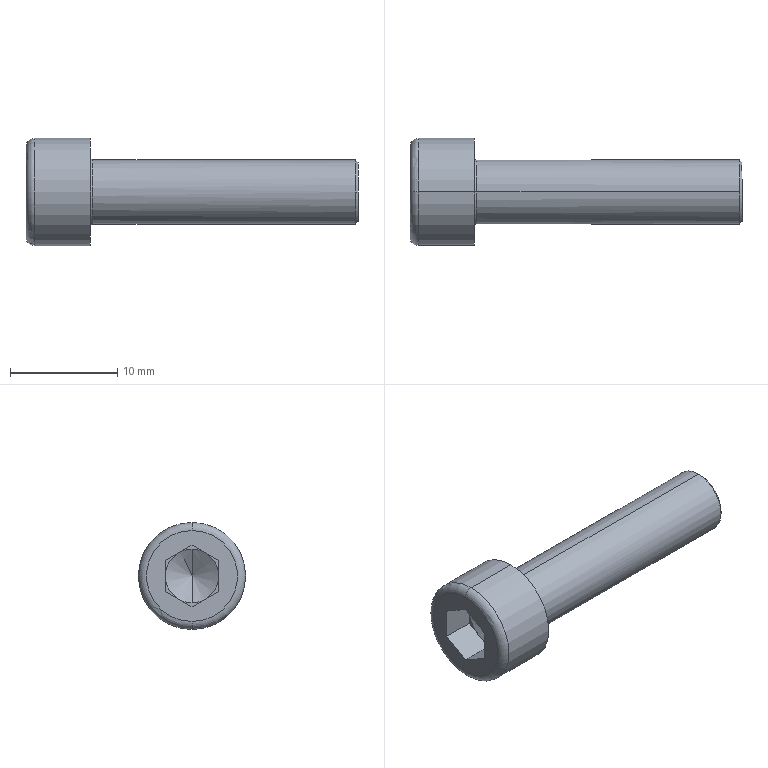Part | SolidWorks | features BaseBody 1 | 1 solid | 27 faces | box 31 x 10 x 10 mm | volume 1100 mm3 | plane 15 | cylinder 4 | cone 4 | torus 4 | commonest cylinder face diameters 6 x2 10 x2
STEP:
#1=CARTESIAN_POINT('',(30.75,3.,0.));
#2=VERTEX_POINT('',#1);
#3=CARTESIAN_POINT('',(30.75,0.,-3.));
#4=VERTEX_POINT('',#3);
#5=CARTESIAN_POINT('',(30.75,0.,0.));
#6=DIRECTION('',(-1.,0.,0.));
#7=DIRECTION('',(0.,0.,1.));
#8=AXIS2_PLACEMENT_3D('',#5,#6,#7);
#9=CIRCLE('',#8,3.);
#10=EDGE_CURVE('',#2,#4,#9,.T.);
#11=ORIENTED_EDGE('',*,*,#10,.T.);
#12=CARTESIAN_POINT('',(6.25,0.,-3.));
#13=VERTEX_POINT('',#12);
#14=CARTESIAN_POINT('',(31.,0.,-3.));
#15=DIRECTION('',(-1.,0.,0.));
#16=VECTOR('',#15,1000.);
#17=LINE('',#14,#16);
#18=EDGE_CURVE('',#4,#13,#17,.T.);
#19=ORIENTED_EDGE('',*,*,#18,.T.);
#20=CARTESIAN_POINT('',(6.25,0.,3.));
#21=VERTEX_POINT('',#20);
#22=CARTESIAN_POINT('',(6.25,0.,0.));
#23=DIRECTION('',(1.,0.,0.));
#24=DIRECTION('',(0.,0.,1.));
#25=AXIS2_PLACEMENT_3D('',#22,#23,#24);
#26=CIRCLE('',#25,3.);
#27=EDGE_CURVE('',#13,#21,#26,.T.);
#28=ORIENTED_EDGE('',*,*,#27,.T.);
#29=CARTESIAN_POINT('',(30.75,0.,3.));
#30=VERTEX_POINT('',#29);
#31=CARTESIAN_POINT('',(31.,0.,3.));
#32=DIRECTION('',(-1.,0.,0.));
#33=VECTOR('',#32,1000.);
#34=LINE('',#31,#33);
#35=EDGE_CURVE('',#30,#21,#34,.T.);
#36=ORIENTED_EDGE('',*,*,#35,.F.);
#37=CARTESIAN_POINT('',(30.75,0.,0.));
#38=DIRECTION('',(-1.,0.,0.));
#39=DIRECTION('',(0.,0.,1.));
#40=AXIS2_PLACEMENT_3D('',#37,#38,#39);
#41=CIRCLE('',#40,3.);
#42=EDGE_CURVE('',#30,#2,#41,.T.);
#43=ORIENTED_EDGE('',*,*,#42,.T.);
#44=EDGE_LOOP('',(#11,#19,#28,#36,#43));
#45=FACE_OUTER_BOUND('',#44,.T.);
#46=CARTESIAN_POINT('',(31.,0.,0.));
#47=DIRECTION('',(-1.,0.,0.));
#48=DIRECTION('',(0.,0.,1.));
#49=AXIS2_PLACEMENT_3D('',#46,#47,#48);
#50=CYLINDRICAL_SURFACE('',#49,3.);
#51=ADVANCED_FACE('',(#45),#50,.T.);
#52=CARTESIAN_POINT('',(31.,-2.75,0.));
#53=VERTEX_POINT('',#52);
#54=CARTESIAN_POINT('',(31.,2.75,0.));
#55=VERTEX_POINT('',#54);
#56=CARTESIAN_POINT('',(31.,0.,0.));
#57=DIRECTION('',(-1.,0.,0.));
#58=DIRECTION('',(0.,-1.,0.));
#59=AXIS2_PLACEMENT_3D('',#56,#57,#58);
#60=CIRCLE('',#59,2.75);
#61=EDGE_CURVE('',#53,#55,#60,.T.);
#62=ORIENTED_EDGE('',*,*,#61,.T.);
#63=CARTESIAN_POINT('',(30.75,3.,0.));
#64=DIRECTION('',(-0.7071,0.7071,0.));
#65=VECTOR('',#64,1000.);
#66=LINE('',#63,#65);
#67=EDGE_CURVE('',#55,#2,#66,.T.);
#68=ORIENTED_EDGE('',*,*,#67,.T.);
#69=ORIENTED_EDGE('',*,*,#42,.F.);
#70=CARTESIAN_POINT('',(30.75,-3.,0.));
#71=VERTEX_POINT('',#70);
#72=CARTESIAN_POINT('',(30.75,0.,0.));
#73=DIRECTION('',(-1.,0.,0.));
#74=DIRECTION('',(0.,0.,1.));
#75=AXIS2_PLACEMENT_3D('',#72,#73,#74);
#76=CIRCLE('',#75,3.);
#77=EDGE_CURVE('',#71,#30,#76,.T.);
#78=ORIENTED_EDGE('',*,*,#77,.F.);
#79=CARTESIAN_POINT('',(30.75,-3.,0.));
#80=DIRECTION('',(-0.7071,-0.7071,0.));
#81=VECTOR('',#80,1000.);
#82=LINE('',#79,#81);
#83=EDGE_CURVE('',#53,#71,#82,.T.);
#84=ORIENTED_EDGE('',*,*,#83,.F.);
#85=EDGE_LOOP('',(#62,#68,#69,#78,#84));
#86=FACE_OUTER_BOUND('',#85,.T.);
#87=CARTESIAN_POINT('',(30.75,0.,0.));
#88=DIRECTION('',(-1.,0.,0.));
#89=DIRECTION('',(0.,-1.,0.));
#90=AXIS2_PLACEMENT_3D('',#87,#88,#89);
#91=CONICAL_SURFACE('',#90,3.,0.7854);
#92=ADVANCED_FACE('',(#86),#91,.T.);
#93=CARTESIAN_POINT('',(6.25,0.,0.));
#94=DIRECTION('',(1.,0.,0.));
#95=DIRECTION('',(0.,0.,1.));
#96=AXIS2_PLACEMENT_3D('',#93,#94,#95);
#97=CIRCLE('',#96,3.);
#98=EDGE_CURVE('',#21,#13,#97,.T.);
#99=ORIENTED_EDGE('',*,*,#98,.F.);
#100=CARTESIAN_POINT('',(6.,0.,3.25));
#101=VERTEX_POINT('',#100);
#102=CARTESIAN_POINT('',(6.25,0.,3.25));
#103=DIRECTION('',(0.,1.,0.));
#104=DIRECTION('',(0.,0.,1.));
#105=AXIS2_PLACEMENT_3D('',#102,#103,#104);
#106=CIRCLE('',#105,0.25);
#107=EDGE_CURVE('',#21,#101,#106,.T.);
#108=ORIENTED_EDGE('',*,*,#107,.T.);
#109=CARTESIAN_POINT('',(6.,0.,-3.25));
#110=VERTEX_POINT('',#109);
#111=CARTESIAN_POINT('',(6.,0.,0.));
#112=DIRECTION('',(-1.,0.,0.));
#113=DIRECTION('',(0.,0.,-1.));
#114=AXIS2_PLACEMENT_3D('',#111,#112,#113);
#115=CIRCLE('',#114,3.25);
#116=EDGE_CURVE('',#110,#101,#115,.T.);
#117=ORIENTED_EDGE('',*,*,#116,.F.);
#118=CARTESIAN_POINT('',(6.25,0.,-3.25));
#119=DIRECTION('',(0.,-1.,0.));
#120=DIRECTION('',(0.,0.,-1.));
#121=AXIS2_PLACEMENT_3D('',#118,#119,#120);
#122=CIRCLE('',#121,0.25);
#123=EDGE_CURVE('',#13,#110,#122,.T.);
#124=ORIENTED_EDGE('',*,*,#123,.F.);
#125=EDGE_LOOP('',(#99,#108,#117,#124));
#126=FACE_OUTER_BOUND('',#125,.T.);
#127=CARTESIAN_POINT('',(6.25,0.,0.));
#128=DIRECTION('',(1.,0.,0.));
#129=DIRECTION('',(0.,0.,-1.));
#130=AXIS2_PLACEMENT_3D('',#127,#128,#129);
#131=TOROIDAL_SURFACE('',#130,3.25,0.25);
#132=ADVANCED_FACE('',(#126),#131,.F.);
#133=CARTESIAN_POINT('',(6.,0.,-5.));
#134=VERTEX_POINT('',#133);
#135=CARTESIAN_POINT('',(6.,0.,5.));
#136=VERTEX_POINT('',#135);
#137=CARTESIAN_POINT('',(6.,0.,0.));
#138=DIRECTION('',(1.,0.,0.));
#139=DIRECTION('',(0.,0.,1.));
#140=AXIS2_PLACEMENT_3D('',#137,#138,#139);
#141=CIRCLE('',#140,5.);
#142=EDGE_CURVE('',#134,#136,#141,.T.);
#143=ORIENTED_EDGE('',*,*,#142,.F.);
#144=CARTESIAN_POINT('',(0.75,0.,-5.));
#145=VERTEX_POINT('',#144);
#146=CARTESIAN_POINT('',(6.,0.,-5.));
#147=DIRECTION('',(-1.,0.,0.));
#148=VECTOR('',#147,1000.);
#149=LINE('',#146,#148);
#150=EDGE_CURVE('',#134,#145,#149,.T.);
#151=ORIENTED_EDGE('',*,*,#150,.T.);
#152=CARTESIAN_POINT('',(0.75,0.,5.));
#153=VERTEX_POINT('',#152);
#154=CARTESIAN_POINT('',(0.75,0.,0.));
#155=DIRECTION('',(1.,0.,0.));
#156=DIRECTION('',(0.,0.,1.));
#157=AXIS2_PLACEMENT_3D('',#154,#155,#156);
#158=CIRCLE('',#157,5.);
#159=EDGE_CURVE('',#145,#153,#158,.T.);
#160=ORIENTED_EDGE('',*,*,#159,.T.);
#161=CARTESIAN_POINT('',(6.,0.,5.));
#162=DIRECTION('',(-1.,0.,0.));
#163=VECTOR('',#162,1000.);
#164=LINE('',#161,#163);
#165=EDGE_CURVE('',#136,#153,#164,.T.);
#166=ORIENTED_EDGE('',*,*,#165,.F.);
#167=EDGE_LOOP('',(#143,#151,#160,#166));
#168=FACE_OUTER_BOUND('',#167,.T.);
#169=CARTESIAN_POINT('',(6.,0.,0.));
#170=DIRECTION('',(-1.,0.,0.));
#171=DIRECTION('',(0.,0.,1.));
#172=AXIS2_PLACEMENT_3D('',#169,#170,#171);
#173=CYLINDRICAL_SURFACE('',#172,5.);
#174=ADVANCED_FACE('',(#168),#173,.T.);
#175=CARTESIAN_POINT('',(0.,0.,-4.25));
#176=VERTEX_POINT('',#175);
#177=CARTESIAN_POINT('',(0.,0.,4.25));
#178=VERTEX_POINT('',#177);
#179=CARTESIAN_POINT('',(0.,0.,0.));
#180=DIRECTION('',(1.,0.,0.));
#181=DIRECTION('',(0.,0.,-1.));
#182=AXIS2_PLACEMENT_3D('',#179,#180,#181);
#183=CIRCLE('',#182,4.25);
#184=EDGE_CURVE('',#176,#178,#183,.T.);
#185=ORIENTED_EDGE('',*,*,#184,.T.);
#186=CARTESIAN_POINT('',(0.75,0.,4.25));
#187=DIRECTION('',(0.,1.,0.));
#188=DIRECTION('',(0.,0.,1.));
#189=AXIS2_PLACEMENT_3D('',#186,#187,#188);
#190=CIRCLE('',#189,0.75);
#191=EDGE_CURVE('',#178,#153,#190,.T.);
#192=ORIENTED_EDGE('',*,*,#191,.T.);
#193=ORIENTED_EDGE('',*,*,#159,.F.);
#194=CARTESIAN_POINT('',(0.75,0.,-4.25));
#195=DIRECTION('',(0.,-1.,0.));
#196=DIRECTION('',(0.,0.,-1.));
#197=AXIS2_PLACEMENT_3D('',#194,#195,#196);
#198=CIRCLE('',#197,0.75);
#199=EDGE_CURVE('',#176,#145,#198,.T.);
#200=ORIENTED_EDGE('',*,*,#199,.F.);
#201=EDGE_LOOP('',(#185,#192,#193,#200));
#202=FACE_OUTER_BOUND('',#201,.T.);
#203=CARTESIAN_POINT('',(0.75,0.,0.));
#204=DIRECTION('',(1.,0.,0.));
#205=DIRECTION('',(0.,0.,-1.));
#206=AXIS2_PLACEMENT_3D('',#203,#204,#205);
#207=TOROIDAL_SURFACE('',#206,4.25,0.75);
#208=ADVANCED_FACE('',(#202),#207,.T.);
#209=CARTESIAN_POINT('',(4.443,0.,0.));
#210=VERTEX_POINT('',#209);
#211=CARTESIAN_POINT('',(3.,0.,2.5));
#212=VERTEX_POINT('',#211);
#213=CARTESIAN_POINT('',(3.,0.,2.5));
#214=DIRECTION('',(-0.5,0.,0.866));
#215=VECTOR('',#214,1000.);
#216=LINE('',#213,#215);
#217=EDGE_CURVE('',#210,#212,#216,.T.);
#218=ORIENTED_EDGE('',*,*,#217,.F.);
#219=CARTESIAN_POINT('',(3.,0.,-2.5));
#220=VERTEX_POINT('',#219);
#221=CARTESIAN_POINT('',(3.,0.,-2.5));
#222=DIRECTION('',(-0.5,0.,-0.866));
#223=VECTOR('',#222,1000.);
#224=LINE('',#221,#223);
#225=EDGE_CURVE('',#210,#220,#224,.T.);
#226=ORIENTED_EDGE('',*,*,#225,.T.);
#227=CARTESIAN_POINT('',(3.,-1.25,-2.165));
#228=VERTEX_POINT('',#227);
#229=CARTESIAN_POINT('',(3.,0.,0.));
#230=DIRECTION('',(1.,0.,0.));
#231=DIRECTION('',(0.,0.,1.));
#232=AXIS2_PLACEMENT_3D('',#229,#230,#231);
#233=CIRCLE('',#232,2.5);
#234=EDGE_CURVE('',#228,#220,#233,.T.);
#235=ORIENTED_EDGE('',*,*,#234,.F.);
#236=CARTESIAN_POINT('',(3.,-2.5,0.));
#237=VERTEX_POINT('',#236);
#238=CARTESIAN_POINT('',(3.,0.,0.));
#239=DIRECTION('',(1.,0.,0.));
#240=DIRECTION('',(0.,0.,1.));
#241=AXIS2_PLACEMENT_3D('',#238,#239,#240);
#242=CIRCLE('',#241,2.5);
#243=EDGE_CURVE('',#237,#228,#242,.T.);
#244=ORIENTED_EDGE('',*,*,#243,.F.);
#245=CARTESIAN_POINT('',(3.,-1.25,2.165));
#246=VERTEX_POINT('',#245);
#247=CARTESIAN_POINT('',(3.,0.,0.));
#248=DIRECTION('',(1.,0.,0.));
#249=DIRECTION('',(0.,0.,1.));
#250=AXIS2_PLACEMENT_3D('',#247,#248,#249);
#251=CIRCLE('',#250,2.5);
#252=EDGE_CURVE('',#246,#237,#251,.T.);
#253=ORIENTED_EDGE('',*,*,#252,.F.);
#254=CARTESIAN_POINT('',(3.,0.,0.));
#255=DIRECTION('',(1.,0.,0.));
#256=DIRECTION('',(0.,0.,1.));
#257=AXIS2_PLACEMENT_3D('',#254,#255,#256);
#258=CIRCLE('',#257,2.5);
#259=EDGE_CURVE('',#212,#246,#258,.T.);
#260=ORIENTED_EDGE('',*,*,#259,.F.);
#261=EDGE_LOOP('',(#218,#226,#235,#244,#253,#260));
#262=FACE_OUTER_BOUND('',#261,.T.);
#263=CARTESIAN_POINT('',(3.,0.,0.));
#264=DIRECTION('',(-1.,0.,0.));
#265=DIRECTION('',(0.,0.,1.));
#266=AXIS2_PLACEMENT_3D('',#263,#264,#265);
#267=CONICAL_SURFACE('',#266,2.5,1.047);
#268=ADVANCED_FACE('',(#262),#267,.F.);
#269=ORIENTED_EDGE('',*,*,#18,.F.);
#270=CARTESIAN_POINT('',(30.75,0.,0.));
#271=DIRECTION('',(-1.,0.,0.));
#272=DIRECTION('',(0.,0.,1.));
#273=AXIS2_PLACEMENT_3D('',#270,#271,#272);
#274=CIRCLE('',#273,3.);
#275=EDGE_CURVE('',#4,#71,#274,.T.);
#276=ORIENTED_EDGE('',*,*,#275,.T.);
#277=ORIENTED_EDGE('',*,*,#77,.T.);
#278=ORIENTED_EDGE('',*,*,#35,.T.);
#279=ORIENTED_EDGE('',*,*,#98,.T.);
#280=EDGE_LOOP('',(#269,#276,#277,#278,#279));
#281=FACE_OUTER_BOUND('',#280,.T.);
#282=CARTESIAN_POINT('',(31.,0.,0.));
#283=DIRECTION('',(-1.,0.,0.));
#284=DIRECTION('',(0.,0.,1.));
#285=AXIS2_PLACEMENT_3D('',#282,#283,#284);
#286=CYLINDRICAL_SURFACE('',#285,3.);
#287=ADVANCED_FACE('',(#281),#286,.T.);
#288=ORIENTED_EDGE('',*,*,#67,.F.);
#289=CARTESIAN_POINT('',(31.,0.,0.));
#290=DIRECTION('',(-1.,0.,0.));
#291=DIRECTION('',(0.,-1.,0.));
#292=AXIS2_PLACEMENT_3D('',#289,#290,#291);
#293=CIRCLE('',#292,2.75);
#294=EDGE_CURVE('',#55,#53,#293,.T.);
#295=ORIENTED_EDGE('',*,*,#294,.T.);
#296=ORIENTED_EDGE('',*,*,#83,.T.);
#297=ORIENTED_EDGE('',*,*,#275,.F.);
#298=ORIENTED_EDGE('',*,*,#10,.F.);
#299=EDGE_LOOP('',(#288,#295,#296,#297,#298));
#300=FACE_OUTER_BOUND('',#299,.T.);
#301=CARTESIAN_POINT('',(30.75,0.,0.));
#302=DIRECTION('',(-1.,0.,0.));
#303=DIRECTION('',(0.,-1.,0.));
#304=AXIS2_PLACEMENT_3D('',#301,#302,#303);
#305=CONICAL_SURFACE('',#304,3.,0.7854);
#306=ADVANCED_FACE('',(#300),#305,.T.);
#307=ORIENTED_EDGE('',*,*,#107,.F.);
#308=ORIENTED_EDGE('',*,*,#27,.F.);
#309=ORIENTED_EDGE('',*,*,#123,.T.);
#310=CARTESIAN_POINT('',(6.,0.,0.));
#311=DIRECTION('',(-1.,0.,0.));
#312=DIRECTION('',(0.,0.,-1.));
#313=AXIS2_PLACEMENT_3D('',#310,#311,#312);
#314=CIRCLE('',#313,3.25);
#315=EDGE_CURVE('',#101,#110,#314,.T.);
#316=ORIENTED_EDGE('',*,*,#315,.F.);
#317=EDGE_LOOP('',(#307,#308,#309,#316));
#318=FACE_OUTER_BOUND('',#317,.T.);
#319=CARTESIAN_POINT('',(6.25,0.,0.));
#320=DIRECTION('',(1.,0.,0.));
#321=DIRECTION('',(0.,0.,-1.));
#322=AXIS2_PLACEMENT_3D('',#319,#320,#321);
#323=TOROIDAL_SURFACE('',#322,3.25,0.25);
#324=ADVANCED_FACE('',(#318),#323,.F.);
#325=ORIENTED_EDGE('',*,*,#61,.F.);
#326=ORIENTED_EDGE('',*,*,#294,.F.);
#327=EDGE_LOOP('',(#325,#326));
#328=FACE_OUTER_BOUND('',#327,.T.);
#329=CARTESIAN_POINT('',(31.,0.,0.));
#330=DIRECTION('',(1.,0.,0.));
#331=DIRECTION('',(0.,0.,-1.));
#332=AXIS2_PLACEMENT_3D('',#329,#330,#331);
#333=PLANE('',#332);
#334=ADVANCED_FACE('',(#328),#333,.T.);
#335=ORIENTED_EDGE('',*,*,#116,.T.);
#336=ORIENTED_EDGE('',*,*,#315,.T.);
#337=EDGE_LOOP('',(#335,#336));
#338=FACE_BOUND('',#337,.T.);
#339=CARTESIAN_POINT('',(6.,0.,0.));
#340=DIRECTION('',(1.,0.,0.));
#341=DIRECTION('',(0.,0.,1.));
#342=AXIS2_PLACEMENT_3D('',#339,#340,#341);
#343=CIRCLE('',#342,5.);
#344=EDGE_CURVE('',#136,#134,#343,.T.);
#345=ORIENTED_EDGE('',*,*,#344,.T.);
#346=ORIENTED_EDGE('',*,*,#142,.T.);
#347=EDGE_LOOP('',(#345,#346));
#348=FACE_OUTER_BOUND('',#347,.T.);
#349=CARTESIAN_POINT('',(6.,0.,0.));
#350=DIRECTION('',(1.,0.,0.));
#351=DIRECTION('',(0.,0.,-1.));
#352=AXIS2_PLACEMENT_3D('',#349,#350,#351);
#353=PLANE('',#352);
#354=ADVANCED_FACE('',(#338,#348),#353,.T.);
#355=ORIENTED_EDGE('',*,*,#150,.F.);
#356=ORIENTED_EDGE('',*,*,#344,.F.);
#357=ORIENTED_EDGE('',*,*,#165,.T.);
#358=CARTESIAN_POINT('',(0.75,0.,0.));
#359=DIRECTION('',(1.,0.,0.));
#360=DIRECTION('',(0.,0.,1.));
#361=AXIS2_PLACEMENT_3D('',#358,#359,#360);
#362=CIRCLE('',#361,5.);
#363=EDGE_CURVE('',#153,#145,#362,.T.);
#364=ORIENTED_EDGE('',*,*,#363,.T.);
#365=EDGE_LOOP('',(#355,#356,#357,#364));
#366=FACE_OUTER_BOUND('',#365,.T.);
#367=CARTESIAN_POINT('',(6.,0.,0.));
#368=DIRECTION('',(-1.,0.,0.));
#369=DIRECTION('',(0.,0.,1.));
#370=AXIS2_PLACEMENT_3D('',#367,#368,#369);
#371=CYLINDRICAL_SURFACE('',#370,5.);
#372=ADVANCED_FACE('',(#366),#371,.T.);
#373=ORIENTED_EDGE('',*,*,#191,.F.);
#374=CARTESIAN_POINT('',(0.,0.,0.));
#375=DIRECTION('',(1.,0.,0.));
#376=DIRECTION('',(0.,0.,-1.));
#377=AXIS2_PLACEMENT_3D('',#374,#375,#376);
#378=CIRCLE('',#377,4.25);
#379=EDGE_CURVE('',#178,#176,#378,.T.);
#380=ORIENTED_EDGE('',*,*,#379,.T.);
#381=ORIENTED_EDGE('',*,*,#199,.T.);
#382=ORIENTED_EDGE('',*,*,#363,.F.);
#383=EDGE_LOOP('',(#373,#380,#381,#382));
#384=FACE_OUTER_BOUND('',#383,.T.);
#385=CARTESIAN_POINT('',(0.75,0.,0.));
#386=DIRECTION('',(1.,0.,0.));
#387=DIRECTION('',(0.,0.,-1.));
#388=AXIS2_PLACEMENT_3D('',#385,#386,#387);
#389=TOROIDAL_SURFACE('',#388,4.25,0.75);
#390=ADVANCED_FACE('',(#384),#389,.T.);
#391=ORIENTED_EDGE('',*,*,#184,.F.);
#392=ORIENTED_EDGE('',*,*,#379,.F.);
#393=EDGE_LOOP('',(#391,#392));
#394=FACE_OUTER_BOUND('',#393,.T.);
#395=CARTESIAN_POINT('',(0.,2.5,1.443));
#396=VERTEX_POINT('',#395);
#397=CARTESIAN_POINT('',(0.,2.5,-1.443));
#398=VERTEX_POINT('',#397);
#399=CARTESIAN_POINT('',(0.,2.5,0.));
#400=DIRECTION('',(0.,0.,-1.));
#401=VECTOR('',#400,1000.);
#402=LINE('',#399,#401);
#403=EDGE_CURVE('',#396,#398,#402,.T.);
#404=ORIENTED_EDGE('',*,*,#403,.F.);
#405=CARTESIAN_POINT('',(0.,0.,2.887));
#406=VERTEX_POINT('',#405);
#407=CARTESIAN_POINT('',(0.,0.,2.887));
#408=DIRECTION('',(0.,0.866,-0.5));
#409=VECTOR('',#408,1000.);
#410=LINE('',#407,#409);
#411=EDGE_CURVE('',#406,#396,#410,.T.);
#412=ORIENTED_EDGE('',*,*,#411,.F.);
#413=CARTESIAN_POINT('',(0.,-2.5,1.443));
#414=VERTEX_POINT('',#413);
#415=CARTESIAN_POINT('',(0.,-2.5,1.443));
#416=DIRECTION('',(0.,0.866,0.5));
#417=VECTOR('',#416,1000.);
#418=LINE('',#415,#417);
#419=EDGE_CURVE('',#414,#406,#418,.T.);
#420=ORIENTED_EDGE('',*,*,#419,.F.);
#421=CARTESIAN_POINT('',(0.,-2.5,-1.443));
#422=VERTEX_POINT('',#421);
#423=CARTESIAN_POINT('',(0.,-2.5,0.));
#424=DIRECTION('',(0.,0.,1.));
#425=VECTOR('',#424,1000.);
#426=LINE('',#423,#425);
#427=EDGE_CURVE('',#422,#414,#426,.T.);
#428=ORIENTED_EDGE('',*,*,#427,.F.);
#429=CARTESIAN_POINT('',(0.,0.,-2.887));
#430=VERTEX_POINT('',#429);
#431=CARTESIAN_POINT('',(0.,0.,-2.887));
#432=DIRECTION('',(0.,-0.866,0.5));
#433=VECTOR('',#432,1000.);
#434=LINE('',#431,#433);
#435=EDGE_CURVE('',#430,#422,#434,.T.);
#436=ORIENTED_EDGE('',*,*,#435,.F.);
#437=CARTESIAN_POINT('',(0.,2.5,-1.443));
#438=DIRECTION('',(0.,-0.866,-0.5));
#439=VECTOR('',#438,1000.);
#440=LINE('',#437,#439);
#441=EDGE_CURVE('',#398,#430,#440,.T.);
#442=ORIENTED_EDGE('',*,*,#441,.F.);
#443=EDGE_LOOP('',(#404,#412,#420,#428,#436,#442));
#444=FACE_BOUND('',#443,.T.);
#445=CARTESIAN_POINT('',(0.,0.,0.));
#446=DIRECTION('',(1.,0.,0.));
#447=DIRECTION('',(0.,0.,-1.));
#448=AXIS2_PLACEMENT_3D('',#445,#446,#447);
#449=PLANE('',#448);
#450=ADVANCED_FACE('',(#394,#444),#449,.F.);
#451=CARTESIAN_POINT('',(3.,0.,-2.887));
#452=VERTEX_POINT('',#451);
#453=CARTESIAN_POINT('',(3.,0.,-2.887));
#454=DIRECTION('',(1.,0.,0.));
#455=VECTOR('',#454,1000.);
#456=LINE('',#453,#455);
#457=EDGE_CURVE('',#430,#452,#456,.T.);
#458=ORIENTED_EDGE('',*,*,#457,.T.);
#459=CARTESIAN_POINT('',(3.,1.25,-2.165));
#460=VERTEX_POINT('',#459);
#461=CARTESIAN_POINT('',(3.,0.,-2.887));
#462=DIRECTION('',(0.,0.866,0.5));
#463=VECTOR('',#462,1000.);
#464=LINE('',#461,#463);
#465=EDGE_CURVE('',#452,#460,#464,.T.);
#466=ORIENTED_EDGE('',*,*,#465,.T.);
#467=CARTESIAN_POINT('',(3.,2.5,-1.443));
#468=VERTEX_POINT('',#467);
#469=CARTESIAN_POINT('',(3.,2.5,-1.443));
#470=DIRECTION('',(0.,-0.866,-0.5));
#471=VECTOR('',#470,1000.);
#472=LINE('',#469,#471);
#473=EDGE_CURVE('',#468,#460,#472,.T.);
#474=ORIENTED_EDGE('',*,*,#473,.F.);
#475=CARTESIAN_POINT('',(3.,2.5,-1.443));
#476=DIRECTION('',(-1.,0.,0.));
#477=VECTOR('',#476,1000.);
#478=LINE('',#475,#477);
#479=EDGE_CURVE('',#468,#398,#478,.T.);
#480=ORIENTED_EDGE('',*,*,#479,.T.);
#481=ORIENTED_EDGE('',*,*,#441,.T.);
#482=EDGE_LOOP('',(#458,#466,#474,#480,#481));
#483=FACE_OUTER_BOUND('',#482,.T.);
#484=CARTESIAN_POINT('',(3.,0.,-2.887));
#485=DIRECTION('',(0.,-0.5,0.866));
#486=DIRECTION('',(0.,-0.866,-0.5));
#487=AXIS2_PLACEMENT_3D('',#484,#485,#486);
#488=PLANE('',#487);
#489=ADVANCED_FACE('',(#483),#488,.T.);
#490=ORIENTED_EDGE('',*,*,#479,.F.);
#491=CARTESIAN_POINT('',(3.,2.5,0.));
#492=VERTEX_POINT('',#491);
#493=CARTESIAN_POINT('',(3.,2.5,0.));
#494=DIRECTION('',(0.,0.,-1.));
#495=VECTOR('',#494,1000.);
#496=LINE('',#493,#495);
#497=EDGE_CURVE('',#492,#468,#496,.T.);
#498=ORIENTED_EDGE('',*,*,#497,.F.);
#499=CARTESIAN_POINT('',(3.,2.5,1.443));
#500=VERTEX_POINT('',#499);
#501=CARTESIAN_POINT('',(3.,2.5,0.));
#502=DIRECTION('',(0.,0.,-1.));
#503=VECTOR('',#502,1000.);
#504=LINE('',#501,#503);
#505=EDGE_CURVE('',#500,#492,#504,.T.);
#506=ORIENTED_EDGE('',*,*,#505,.F.);
#507=CARTESIAN_POINT('',(3.,2.5,1.443));
#508=DIRECTION('',(-1.,0.,0.));
#509=VECTOR('',#508,1000.);
#510=LINE('',#507,#509);
#511=EDGE_CURVE('',#500,#396,#510,.T.);
#512=ORIENTED_EDGE('',*,*,#511,.T.);
#513=ORIENTED_EDGE('',*,*,#403,.T.);
#514=EDGE_LOOP('',(#490,#498,#506,#512,#513));
#515=FACE_OUTER_BOUND('',#514,.T.);
#516=CARTESIAN_POINT('',(3.,2.5,-1.443));
#517=DIRECTION('',(0.,-1.,0.));
#518=DIRECTION('',(0.,0.,-1.));
#519=AXIS2_PLACEMENT_3D('',#516,#517,#518);
#520=PLANE('',#519);
#521=ADVANCED_FACE('',(#515),#520,.T.);
#522=ORIENTED_EDGE('',*,*,#511,.F.);
#523=CARTESIAN_POINT('',(3.,1.25,2.165));
#524=VERTEX_POINT('',#523);
#525=CARTESIAN_POINT('',(3.,1.25,2.165));
#526=DIRECTION('',(0.,0.866,-0.5));
#527=VECTOR('',#526,1000.);
#528=LINE('',#525,#527);
#529=EDGE_CURVE('',#524,#500,#528,.T.);
#530=ORIENTED_EDGE('',*,*,#529,.F.);
#531=CARTESIAN_POINT('',(3.,0.,2.887));
#532=VERTEX_POINT('',#531);
#533=CARTESIAN_POINT('',(3.,2.5,1.443));
#534=DIRECTION('',(0.,-0.866,0.5));
#535=VECTOR('',#534,1000.);
#536=LINE('',#533,#535);
#537=EDGE_CURVE('',#524,#532,#536,.T.);
#538=ORIENTED_EDGE('',*,*,#537,.T.);
#539=CARTESIAN_POINT('',(3.,0.,2.887));
#540=DIRECTION('',(-1.,0.,0.));
#541=VECTOR('',#540,1000.);
#542=LINE('',#539,#541);
#543=EDGE_CURVE('',#532,#406,#542,.T.);
#544=ORIENTED_EDGE('',*,*,#543,.T.);
#545=ORIENTED_EDGE('',*,*,#411,.T.);
#546=EDGE_LOOP('',(#522,#530,#538,#544,#545));
#547=FACE_OUTER_BOUND('',#546,.T.);
#548=CARTESIAN_POINT('',(3.,2.5,1.443));
#549=DIRECTION('',(0.,-0.5,-0.866));
#550=DIRECTION('',(0.,0.866,-0.5));
#551=AXIS2_PLACEMENT_3D('',#548,#549,#550);
#552=PLANE('',#551);
#553=ADVANCED_FACE('',(#547),#552,.T.);
#554=ORIENTED_EDGE('',*,*,#543,.F.);
#555=CARTESIAN_POINT('',(3.,0.,2.887));
#556=DIRECTION('',(0.,-0.866,-0.5));
#557=VECTOR('',#556,1000.);
#558=LINE('',#555,#557);
#559=EDGE_CURVE('',#532,#246,#558,.T.);
#560=ORIENTED_EDGE('',*,*,#559,.T.);
#561=CARTESIAN_POINT('',(3.,-2.5,1.443));
#562=VERTEX_POINT('',#561);
#563=CARTESIAN_POINT('',(3.,-2.5,1.443));
#564=DIRECTION('',(0.,0.866,0.5));
#565=VECTOR('',#564,1000.);
#566=LINE('',#563,#565);
#567=EDGE_CURVE('',#562,#246,#566,.T.);
#568=ORIENTED_EDGE('',*,*,#567,.F.);
#569=CARTESIAN_POINT('',(3.,-2.5,1.443));
#570=DIRECTION('',(-1.,0.,0.));
#571=VECTOR('',#570,1000.);
#572=LINE('',#569,#571);
#573=EDGE_CURVE('',#562,#414,#572,.T.);
#574=ORIENTED_EDGE('',*,*,#573,.T.);
#575=ORIENTED_EDGE('',*,*,#419,.T.);
#576=EDGE_LOOP('',(#554,#560,#568,#574,#575));
#577=FACE_OUTER_BOUND('',#576,.T.);
#578=CARTESIAN_POINT('',(3.,0.,2.887));
#579=DIRECTION('',(0.,0.5,-0.866));
#580=DIRECTION('',(0.,0.866,0.5));
#581=AXIS2_PLACEMENT_3D('',#578,#579,#580);
#582=PLANE('',#581);
#583=ADVANCED_FACE('',(#577),#582,.T.);
#584=ORIENTED_EDGE('',*,*,#573,.F.);
#585=CARTESIAN_POINT('',(3.,-2.5,0.));
#586=DIRECTION('',(0.,0.,1.));
#587=VECTOR('',#586,1000.);
#588=LINE('',#585,#587);
#589=EDGE_CURVE('',#237,#562,#588,.T.);
#590=ORIENTED_EDGE('',*,*,#589,.F.);
#591=CARTESIAN_POINT('',(3.,-2.5,-1.443));
#592=VERTEX_POINT('',#591);
#593=CARTESIAN_POINT('',(3.,-2.5,1.443));
#594=DIRECTION('',(0.,0.,-1.));
#595=VECTOR('',#594,1000.);
#596=LINE('',#593,#595);
#597=EDGE_CURVE('',#237,#592,#596,.T.);
#598=ORIENTED_EDGE('',*,*,#597,.T.);
#599=CARTESIAN_POINT('',(3.,-2.5,-1.443));
#600=DIRECTION('',(-1.,0.,0.));
#601=VECTOR('',#600,1000.);
#602=LINE('',#599,#601);
#603=EDGE_CURVE('',#592,#422,#602,.T.);
#604=ORIENTED_EDGE('',*,*,#603,.T.);
#605=ORIENTED_EDGE('',*,*,#427,.T.);
#606=EDGE_LOOP('',(#584,#590,#598,#604,#605));
#607=FACE_OUTER_BOUND('',#606,.T.);
#608=CARTESIAN_POINT('',(3.,-2.5,1.443));
#609=DIRECTION('',(0.,1.,0.));
#610=DIRECTION('',(0.,0.,1.));
#611=AXIS2_PLACEMENT_3D('',#608,#609,#610);
#612=PLANE('',#611);
#613=ADVANCED_FACE('',(#607),#612,.T.);
#614=ORIENTED_EDGE('',*,*,#603,.F.);
#615=CARTESIAN_POINT('',(3.,-2.5,-1.443));
#616=DIRECTION('',(0.,0.866,-0.5));
#617=VECTOR('',#616,1000.);
#618=LINE('',#615,#617);
#619=EDGE_CURVE('',#592,#228,#618,.T.);
#620=ORIENTED_EDGE('',*,*,#619,.T.);
#621=CARTESIAN_POINT('',(3.,-2.5,-1.443));
#622=DIRECTION('',(0.,0.866,-0.5));
#623=VECTOR('',#622,1000.);
#624=LINE('',#621,#623);
#625=EDGE_CURVE('',#228,#452,#624,.T.);
#626=ORIENTED_EDGE('',*,*,#625,.T.);
#627=ORIENTED_EDGE('',*,*,#457,.F.);
#628=ORIENTED_EDGE('',*,*,#435,.T.);
#629=EDGE_LOOP('',(#614,#620,#626,#627,#628));
#630=FACE_OUTER_BOUND('',#629,.T.);
#631=CARTESIAN_POINT('',(3.,-2.5,-1.443));
#632=DIRECTION('',(0.,0.5,0.866));
#633=DIRECTION('',(0.,-0.866,0.5));
#634=AXIS2_PLACEMENT_3D('',#631,#632,#633);
#635=PLANE('',#634);
#636=ADVANCED_FACE('',(#630),#635,.T.);
#637=ORIENTED_EDGE('',*,*,#465,.F.);
#638=ORIENTED_EDGE('',*,*,#625,.F.);
#639=ORIENTED_EDGE('',*,*,#234,.T.);
#640=CARTESIAN_POINT('',(3.,0.,0.));
#641=DIRECTION('',(1.,0.,0.));
#642=DIRECTION('',(0.,0.,1.));
#643=AXIS2_PLACEMENT_3D('',#640,#641,#642);
#644=CIRCLE('',#643,2.5);
#645=EDGE_CURVE('',#220,#460,#644,.T.);
#646=ORIENTED_EDGE('',*,*,#645,.T.);
#647=EDGE_LOOP('',(#637,#638,#639,#646));
#648=FACE_OUTER_BOUND('',#647,.T.);
#649=CARTESIAN_POINT('',(3.,-5.,0.));
#650=DIRECTION('',(-1.,0.,0.));
#651=DIRECTION('',(0.,0.,1.));
#652=AXIS2_PLACEMENT_3D('',#649,#650,#651);
#653=PLANE('',#652);
#654=ADVANCED_FACE('',(#648),#653,.T.);
#655=ORIENTED_EDGE('',*,*,#559,.F.);
#656=ORIENTED_EDGE('',*,*,#537,.F.);
#657=CARTESIAN_POINT('',(3.,0.,0.));
#658=DIRECTION('',(1.,0.,0.));
#659=DIRECTION('',(0.,0.,1.));
#660=AXIS2_PLACEMENT_3D('',#657,#658,#659);
#661=CIRCLE('',#660,2.5);
#662=EDGE_CURVE('',#524,#212,#661,.T.);
#663=ORIENTED_EDGE('',*,*,#662,.T.);
#664=ORIENTED_EDGE('',*,*,#259,.T.);
#665=EDGE_LOOP('',(#655,#656,#663,#664));
#666=FACE_OUTER_BOUND('',#665,.T.);
#667=CARTESIAN_POINT('',(3.,-5.,0.));
#668=DIRECTION('',(-1.,0.,0.));
#669=DIRECTION('',(0.,0.,1.));
#670=AXIS2_PLACEMENT_3D('',#667,#668,#669);
#671=PLANE('',#670);
#672=ADVANCED_FACE('',(#666),#671,.T.);
#673=ORIENTED_EDGE('',*,*,#619,.F.);
#674=ORIENTED_EDGE('',*,*,#597,.F.);
#675=ORIENTED_EDGE('',*,*,#243,.T.);
#676=EDGE_LOOP('',(#673,#674,#675));
#677=FACE_OUTER_BOUND('',#676,.T.);
#678=CARTESIAN_POINT('',(3.,-5.,0.));
#679=DIRECTION('',(-1.,0.,0.));
#680=DIRECTION('',(0.,0.,1.));
#681=AXIS2_PLACEMENT_3D('',#678,#679,#680);
#682=PLANE('',#681);
#683=ADVANCED_FACE('',(#677),#682,.T.);
#684=ORIENTED_EDGE('',*,*,#225,.F.);
#685=ORIENTED_EDGE('',*,*,#217,.T.);
#686=ORIENTED_EDGE('',*,*,#662,.F.);
#687=CARTESIAN_POINT('',(3.,0.,0.));
#688=DIRECTION('',(1.,0.,0.));
#689=DIRECTION('',(0.,0.,1.));
#690=AXIS2_PLACEMENT_3D('',#687,#688,#689);
#691=CIRCLE('',#690,2.5);
#692=EDGE_CURVE('',#492,#524,#691,.T.);
#693=ORIENTED_EDGE('',*,*,#692,.F.);
#694=CARTESIAN_POINT('',(3.,0.,0.));
#695=DIRECTION('',(1.,0.,0.));
#696=DIRECTION('',(0.,0.,1.));
#697=AXIS2_PLACEMENT_3D('',#694,#695,#696);
#698=CIRCLE('',#697,2.5);
#699=EDGE_CURVE('',#460,#492,#698,.T.);
#700=ORIENTED_EDGE('',*,*,#699,.F.);
#701=ORIENTED_EDGE('',*,*,#645,.F.);
#702=EDGE_LOOP('',(#684,#685,#686,#693,#700,#701));
#703=FACE_OUTER_BOUND('',#702,.T.);
#704=CARTESIAN_POINT('',(3.,0.,0.));
#705=DIRECTION('',(-1.,0.,0.));
#706=DIRECTION('',(0.,0.,1.));
#707=AXIS2_PLACEMENT_3D('',#704,#705,#706);
#708=CONICAL_SURFACE('',#707,2.5,1.047);
#709=ADVANCED_FACE('',(#703),#708,.F.);
#710=ORIENTED_EDGE('',*,*,#589,.T.);
#711=ORIENTED_EDGE('',*,*,#567,.T.);
#712=ORIENTED_EDGE('',*,*,#252,.T.);
#713=EDGE_LOOP('',(#710,#711,#712));
#714=FACE_OUTER_BOUND('',#713,.T.);
#715=CARTESIAN_POINT('',(3.,-5.,0.));
#716=DIRECTION('',(-1.,0.,0.));
#717=DIRECTION('',(0.,0.,1.));
#718=AXIS2_PLACEMENT_3D('',#715,#716,#717);
#719=PLANE('',#718);
#720=ADVANCED_FACE('',(#714),#719,.T.);
#721=ORIENTED_EDGE('',*,*,#529,.T.);
#722=ORIENTED_EDGE('',*,*,#505,.T.);
#723=ORIENTED_EDGE('',*,*,#692,.T.);
#724=EDGE_LOOP('',(#721,#722,#723));
#725=FACE_OUTER_BOUND('',#724,.T.);
#726=CARTESIAN_POINT('',(3.,-5.,0.));
#727=DIRECTION('',(-1.,0.,0.));
#728=DIRECTION('',(0.,0.,1.));
#729=AXIS2_PLACEMENT_3D('',#726,#727,#728);
#730=PLANE('',#729);
#731=ADVANCED_FACE('',(#725),#730,.T.);
#732=ORIENTED_EDGE('',*,*,#497,.T.);
#733=ORIENTED_EDGE('',*,*,#473,.T.);
#734=ORIENTED_EDGE('',*,*,#699,.T.);
#735=EDGE_LOOP('',(#732,#733,#734));
#736=FACE_OUTER_BOUND('',#735,.T.);
#737=CARTESIAN_POINT('',(3.,-5.,0.));
#738=DIRECTION('',(-1.,0.,0.));
#739=DIRECTION('',(0.,0.,1.));
#740=AXIS2_PLACEMENT_3D('',#737,#738,#739);
#741=PLANE('',#740);
#742=ADVANCED_FACE('',(#736),#741,.T.);
#743=CLOSED_SHELL('',(#51,#92,#132,#174,#208,#268,#287,#306,#324,#334,#354,#372,#390,#450,#489,#521,#553,#583,#613,#636,#654,#672,#683,#709,#720,#731,#742));
#744=MANIFOLD_SOLID_BREP('',#743);
#745=CARTESIAN_POINT('',(0.,0.,0.));
#746=DIRECTION('',(0.,0.,1.));
#747=DIRECTION('',(1.,0.,0.));
#748=AXIS2_PLACEMENT_3D('',#745,#746,#747);
#749=(LENGTH_UNIT()NAMED_UNIT(*)SI_UNIT(.MILLI.,.METRE.));
#750=UNCERTAINTY_MEASURE_WITH_UNIT(LENGTH_MEASURE(0.00001),#749,'','');
#751=(NAMED_UNIT(*)PLANE_ANGLE_UNIT()SI_UNIT($,.RADIAN.));
#752=(NAMED_UNIT(*)SI_UNIT($,.STERADIAN.)SOLID_ANGLE_UNIT());
#753=(GEOMETRIC_REPRESENTATION_CONTEXT(3)GLOBAL_UNCERTAINTY_ASSIGNED_CONTEXT((#750))GLOBAL_UNIT_ASSIGNED_CONTEXT((#749,#751,#752))REPRESENTATION_CONTEXT('',''));
#754=ADVANCED_BREP_SHAPE_REPRESENTATION('',(#744,#748),#753);